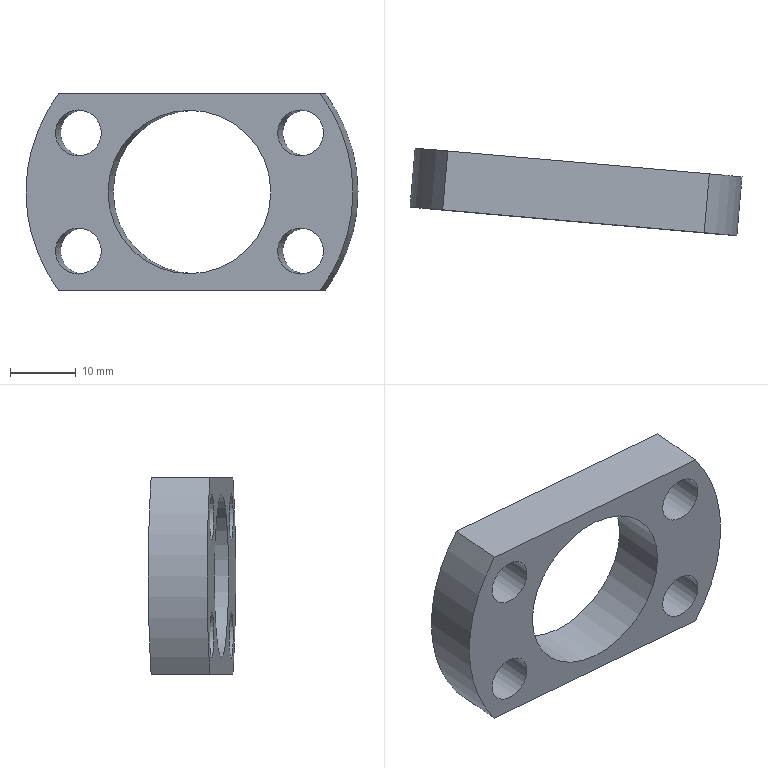Part | NX | features solid 2 | 1 solid | 11 faces | box 50.594 x 13.324 x 30 mm | volume 6871 mm3 | cylinder 7 | plane 4 | commonest cylinder face diameters 7 x4 50 x2 24.9 x1
STEP:
#1=CARTESIAN_POINT('',(318.521,-30.878,-100.));
#2=VERTEX_POINT('',#1);
#3=CARTESIAN_POINT('',(318.521,-30.878,-70.));
#4=VERTEX_POINT('',#3);
#5=CARTESIAN_POINT('',(298.597,-29.135,-85.));
#6=DIRECTION('',(-0.08716,-0.9962,0.));
#7=DIRECTION('',(-0.9962,0.08716,0.));
#8=AXIS2_PLACEMENT_3D('',#5,#6,#7);
#9=CIRCLE('',#8,25.);
#10=EDGE_CURVE('',#2,#4,#9,.T.);
#11=ORIENTED_EDGE('',*,*,#10,.T.);
#12=CARTESIAN_POINT('',(317.736,-39.844,-70.));
#13=VERTEX_POINT('',#12);
#14=CARTESIAN_POINT('',(318.521,-30.878,-70.));
#15=DIRECTION('',(-0.08716,-0.9962,0.));
#16=VECTOR('',#15,1000.);
#17=LINE('',#14,#16);
#18=EDGE_CURVE('',#4,#13,#17,.T.);
#19=ORIENTED_EDGE('',*,*,#18,.T.);
#20=CARTESIAN_POINT('',(317.736,-39.844,-100.));
#21=VERTEX_POINT('',#20);
#22=CARTESIAN_POINT('',(297.813,-38.101,-85.));
#23=DIRECTION('',(-0.08716,-0.9962,0.));
#24=DIRECTION('',(-0.9962,0.08716,0.));
#25=AXIS2_PLACEMENT_3D('',#22,#23,#24);
#26=CIRCLE('',#25,25.);
#27=EDGE_CURVE('',#21,#13,#26,.T.);
#28=ORIENTED_EDGE('',*,*,#27,.F.);
#29=CARTESIAN_POINT('',(318.521,-30.878,-100.));
#30=DIRECTION('',(-0.08716,-0.9962,0.));
#31=VECTOR('',#30,1000.);
#32=LINE('',#29,#31);
#33=EDGE_CURVE('',#2,#21,#32,.T.);
#34=ORIENTED_EDGE('',*,*,#33,.F.);
#35=EDGE_LOOP('',(#11,#19,#28,#34));
#36=FACE_BOUND('',#35,.T.);
#37=CARTESIAN_POINT('',(298.597,-29.135,-85.));
#38=DIRECTION('',(-0.08716,-0.9962,0.));
#39=DIRECTION('',(0.,0.,-1.));
#40=AXIS2_PLACEMENT_3D('',#37,#38,#39);
#41=CYLINDRICAL_SURFACE('',#40,25.);
#42=ADVANCED_FACE('',(#36),#41,.T.);
#43=CARTESIAN_POINT('',(277.889,-36.358,-70.));
#44=VERTEX_POINT('',#43);
#45=CARTESIAN_POINT('',(277.889,-36.358,-100.));
#46=VERTEX_POINT('',#45);
#47=CARTESIAN_POINT('',(297.813,-38.101,-85.));
#48=DIRECTION('',(-0.08716,-0.9962,0.));
#49=DIRECTION('',(-0.9962,0.08716,0.));
#50=AXIS2_PLACEMENT_3D('',#47,#48,#49);
#51=CIRCLE('',#50,25.);
#52=EDGE_CURVE('',#44,#46,#51,.T.);
#53=ORIENTED_EDGE('',*,*,#52,.F.);
#54=CARTESIAN_POINT('',(278.673,-27.392,-70.));
#55=VERTEX_POINT('',#54);
#56=CARTESIAN_POINT('',(278.673,-27.392,-70.));
#57=DIRECTION('',(-0.08716,-0.9962,0.));
#58=VECTOR('',#57,1000.);
#59=LINE('',#56,#58);
#60=EDGE_CURVE('',#44,#55,#59,.F.);
#61=ORIENTED_EDGE('',*,*,#60,.T.);
#62=CARTESIAN_POINT('',(278.673,-27.392,-100.));
#63=VERTEX_POINT('',#62);
#64=CARTESIAN_POINT('',(298.597,-29.135,-85.));
#65=DIRECTION('',(-0.08716,-0.9962,0.));
#66=DIRECTION('',(-0.9962,0.08716,0.));
#67=AXIS2_PLACEMENT_3D('',#64,#65,#66);
#68=CIRCLE('',#67,25.);
#69=EDGE_CURVE('',#55,#63,#68,.T.);
#70=ORIENTED_EDGE('',*,*,#69,.T.);
#71=CARTESIAN_POINT('',(278.673,-27.392,-100.));
#72=DIRECTION('',(-0.08716,-0.9962,0.));
#73=VECTOR('',#72,1000.);
#74=LINE('',#71,#73);
#75=EDGE_CURVE('',#46,#63,#74,.F.);
#76=ORIENTED_EDGE('',*,*,#75,.F.);
#77=EDGE_LOOP('',(#53,#61,#70,#76));
#78=FACE_BOUND('',#77,.T.);
#79=CARTESIAN_POINT('',(298.597,-29.135,-85.));
#80=DIRECTION('',(-0.08716,-0.9962,0.));
#81=DIRECTION('',(0.,0.,-1.));
#82=AXIS2_PLACEMENT_3D('',#79,#80,#81);
#83=CYLINDRICAL_SURFACE('',#82,25.);
#84=ADVANCED_FACE('',(#78),#83,.T.);
#85=CARTESIAN_POINT('',(315.532,-30.617,-90.5));
#86=VERTEX_POINT('',#85);
#87=CARTESIAN_POINT('',(315.532,-30.617,-94.));
#88=DIRECTION('',(-0.08716,-0.9962,0.));
#89=DIRECTION('',(0.,0.,1.));
#90=AXIS2_PLACEMENT_3D('',#87,#88,#89);
#91=CIRCLE('',#90,3.5);
#92=EDGE_CURVE('',#86,#86,#91,.T.);
#93=ORIENTED_EDGE('',*,*,#92,.T.);
#94=EDGE_LOOP('',(#93));
#95=FACE_BOUND('',#94,.T.);
#96=CARTESIAN_POINT('',(315.532,-30.617,-72.5));
#97=VERTEX_POINT('',#96);
#98=CARTESIAN_POINT('',(315.532,-30.617,-76.));
#99=DIRECTION('',(-0.08716,-0.9962,0.));
#100=DIRECTION('',(0.,0.,1.));
#101=AXIS2_PLACEMENT_3D('',#98,#99,#100);
#102=CIRCLE('',#101,3.5);
#103=EDGE_CURVE('',#97,#97,#102,.T.);
#104=ORIENTED_EDGE('',*,*,#103,.T.);
#105=EDGE_LOOP('',(#104));
#106=FACE_BOUND('',#105,.T.);
#107=CARTESIAN_POINT('',(281.662,-27.654,-90.5));
#108=VERTEX_POINT('',#107);
#109=CARTESIAN_POINT('',(281.662,-27.654,-94.));
#110=DIRECTION('',(-0.08716,-0.9962,0.));
#111=DIRECTION('',(0.,0.,1.));
#112=AXIS2_PLACEMENT_3D('',#109,#110,#111);
#113=CIRCLE('',#112,3.5);
#114=EDGE_CURVE('',#108,#108,#113,.T.);
#115=ORIENTED_EDGE('',*,*,#114,.T.);
#116=EDGE_LOOP('',(#115));
#117=FACE_BOUND('',#116,.T.);
#118=CARTESIAN_POINT('',(281.662,-27.654,-72.5));
#119=VERTEX_POINT('',#118);
#120=CARTESIAN_POINT('',(281.662,-27.654,-76.));
#121=DIRECTION('',(-0.08716,-0.9962,0.));
#122=DIRECTION('',(0.,0.,1.));
#123=AXIS2_PLACEMENT_3D('',#120,#121,#122);
#124=CIRCLE('',#123,3.5);
#125=EDGE_CURVE('',#119,#119,#124,.T.);
#126=ORIENTED_EDGE('',*,*,#125,.T.);
#127=EDGE_LOOP('',(#126));
#128=FACE_BOUND('',#127,.T.);
#129=CARTESIAN_POINT('',(298.597,-29.135,-72.55));
#130=VERTEX_POINT('',#129);
#131=CARTESIAN_POINT('',(298.597,-29.135,-85.));
#132=DIRECTION('',(-0.08716,-0.9962,0.));
#133=DIRECTION('',(0.,0.,1.));
#134=AXIS2_PLACEMENT_3D('',#131,#132,#133);
#135=CIRCLE('',#134,12.45);
#136=EDGE_CURVE('',#130,#130,#135,.T.);
#137=ORIENTED_EDGE('',*,*,#136,.T.);
#138=EDGE_LOOP('',(#137));
#139=FACE_BOUND('',#138,.T.);
#140=ORIENTED_EDGE('',*,*,#69,.F.);
#141=CARTESIAN_POINT('',(298.597,-29.135,-70.));
#142=DIRECTION('',(-0.9962,0.08716,0.));
#143=VECTOR('',#142,1000.);
#144=LINE('',#141,#143);
#145=EDGE_CURVE('',#4,#55,#144,.T.);
#146=ORIENTED_EDGE('',*,*,#145,.F.);
#147=ORIENTED_EDGE('',*,*,#10,.F.);
#148=CARTESIAN_POINT('',(298.597,-29.135,-100.));
#149=DIRECTION('',(-0.9962,0.08716,0.));
#150=VECTOR('',#149,1000.);
#151=LINE('',#148,#150);
#152=EDGE_CURVE('',#2,#63,#151,.T.);
#153=ORIENTED_EDGE('',*,*,#152,.T.);
#154=EDGE_LOOP('',(#140,#146,#147,#153));
#155=FACE_BOUND('',#154,.T.);
#156=CARTESIAN_POINT('',(298.597,-29.135,-85.));
#157=DIRECTION('',(0.08716,0.9962,0.));
#158=DIRECTION('',(0.,0.,1.));
#159=AXIS2_PLACEMENT_3D('',#156,#157,#158);
#160=PLANE('',#159);
#161=ADVANCED_FACE('',(#95,#106,#117,#128,#139,#155),#160,.T.);
#162=CARTESIAN_POINT('',(314.748,-39.583,-90.5));
#163=VERTEX_POINT('',#162);
#164=CARTESIAN_POINT('',(314.748,-39.583,-94.));
#165=DIRECTION('',(-0.08716,-0.9962,0.));
#166=DIRECTION('',(0.,0.,1.));
#167=AXIS2_PLACEMENT_3D('',#164,#165,#166);
#168=CIRCLE('',#167,3.5);
#169=EDGE_CURVE('',#163,#163,#168,.T.);
#170=ORIENTED_EDGE('',*,*,#169,.F.);
#171=EDGE_LOOP('',(#170));
#172=FACE_BOUND('',#171,.T.);
#173=CARTESIAN_POINT('',(314.748,-39.583,-72.5));
#174=VERTEX_POINT('',#173);
#175=CARTESIAN_POINT('',(314.748,-39.583,-76.));
#176=DIRECTION('',(-0.08716,-0.9962,0.));
#177=DIRECTION('',(0.,0.,1.));
#178=AXIS2_PLACEMENT_3D('',#175,#176,#177);
#179=CIRCLE('',#178,3.5);
#180=EDGE_CURVE('',#174,#174,#179,.T.);
#181=ORIENTED_EDGE('',*,*,#180,.F.);
#182=EDGE_LOOP('',(#181));
#183=FACE_BOUND('',#182,.T.);
#184=CARTESIAN_POINT('',(280.877,-36.619,-90.5));
#185=VERTEX_POINT('',#184);
#186=CARTESIAN_POINT('',(280.877,-36.619,-94.));
#187=DIRECTION('',(-0.08716,-0.9962,0.));
#188=DIRECTION('',(0.,0.,1.));
#189=AXIS2_PLACEMENT_3D('',#186,#187,#188);
#190=CIRCLE('',#189,3.5);
#191=EDGE_CURVE('',#185,#185,#190,.T.);
#192=ORIENTED_EDGE('',*,*,#191,.F.);
#193=EDGE_LOOP('',(#192));
#194=FACE_BOUND('',#193,.T.);
#195=CARTESIAN_POINT('',(280.877,-36.619,-72.5));
#196=VERTEX_POINT('',#195);
#197=CARTESIAN_POINT('',(280.877,-36.619,-76.));
#198=DIRECTION('',(-0.08716,-0.9962,0.));
#199=DIRECTION('',(0.,0.,1.));
#200=AXIS2_PLACEMENT_3D('',#197,#198,#199);
#201=CIRCLE('',#200,3.5);
#202=EDGE_CURVE('',#196,#196,#201,.T.);
#203=ORIENTED_EDGE('',*,*,#202,.F.);
#204=EDGE_LOOP('',(#203));
#205=FACE_BOUND('',#204,.T.);
#206=CARTESIAN_POINT('',(297.813,-38.101,-72.55));
#207=VERTEX_POINT('',#206);
#208=CARTESIAN_POINT('',(297.813,-38.101,-85.));
#209=DIRECTION('',(-0.08716,-0.9962,0.));
#210=DIRECTION('',(0.,0.,1.));
#211=AXIS2_PLACEMENT_3D('',#208,#209,#210);
#212=CIRCLE('',#211,12.45);
#213=EDGE_CURVE('',#207,#207,#212,.T.);
#214=ORIENTED_EDGE('',*,*,#213,.F.);
#215=EDGE_LOOP('',(#214));
#216=FACE_BOUND('',#215,.T.);
#217=ORIENTED_EDGE('',*,*,#27,.T.);
#218=CARTESIAN_POINT('',(297.813,-38.101,-70.));
#219=DIRECTION('',(-0.9962,0.08716,0.));
#220=VECTOR('',#219,1000.);
#221=LINE('',#218,#220);
#222=EDGE_CURVE('',#13,#44,#221,.T.);
#223=ORIENTED_EDGE('',*,*,#222,.T.);
#224=ORIENTED_EDGE('',*,*,#52,.T.);
#225=CARTESIAN_POINT('',(297.813,-38.101,-100.));
#226=DIRECTION('',(-0.9962,0.08716,0.));
#227=VECTOR('',#226,1000.);
#228=LINE('',#225,#227);
#229=EDGE_CURVE('',#21,#46,#228,.T.);
#230=ORIENTED_EDGE('',*,*,#229,.F.);
#231=EDGE_LOOP('',(#217,#223,#224,#230));
#232=FACE_BOUND('',#231,.T.);
#233=CARTESIAN_POINT('',(297.813,-38.101,-85.));
#234=DIRECTION('',(0.08716,0.9962,0.));
#235=DIRECTION('',(0.,0.,1.));
#236=AXIS2_PLACEMENT_3D('',#233,#234,#235);
#237=PLANE('',#236);
#238=ADVANCED_FACE('',(#172,#183,#194,#205,#216,#232),#237,.F.);
#239=ORIENTED_EDGE('',*,*,#145,.T.);
#240=ORIENTED_EDGE('',*,*,#60,.F.);
#241=ORIENTED_EDGE('',*,*,#222,.F.);
#242=ORIENTED_EDGE('',*,*,#18,.F.);
#243=EDGE_LOOP('',(#239,#240,#241,#242));
#244=FACE_BOUND('',#243,.T.);
#245=CARTESIAN_POINT('',(385.07,-45.735,-70.));
#246=DIRECTION('',(0.,0.,1.));
#247=DIRECTION('',(-0.9962,0.08716,0.));
#248=AXIS2_PLACEMENT_3D('',#245,#246,#247);
#249=PLANE('',#248);
#250=ADVANCED_FACE('',(#244),#249,.T.);
#251=ORIENTED_EDGE('',*,*,#152,.F.);
#252=ORIENTED_EDGE('',*,*,#33,.T.);
#253=ORIENTED_EDGE('',*,*,#229,.T.);
#254=ORIENTED_EDGE('',*,*,#75,.T.);
#255=EDGE_LOOP('',(#251,#252,#253,#254));
#256=FACE_BOUND('',#255,.T.);
#257=CARTESIAN_POINT('',(385.07,-45.735,-100.));
#258=DIRECTION('',(0.,0.,1.));
#259=DIRECTION('',(-0.9962,0.08716,0.));
#260=AXIS2_PLACEMENT_3D('',#257,#258,#259);
#261=PLANE('',#260);
#262=ADVANCED_FACE('',(#256),#261,.F.);
#263=ORIENTED_EDGE('',*,*,#136,.F.);
#264=EDGE_LOOP('',(#263));
#265=FACE_BOUND('',#264,.T.);
#266=ORIENTED_EDGE('',*,*,#213,.T.);
#267=EDGE_LOOP('',(#266));
#268=FACE_BOUND('',#267,.T.);
#269=CARTESIAN_POINT('',(264.432,-419.644,-85.));
#270=DIRECTION('',(0.08716,0.9962,0.));
#271=DIRECTION('',(0.,0.,1.));
#272=AXIS2_PLACEMENT_3D('',#269,#270,#271);
#273=CYLINDRICAL_SURFACE('',#272,12.45);
#274=ADVANCED_FACE('',(#265,#268),#273,.F.);
#275=ORIENTED_EDGE('',*,*,#125,.F.);
#276=EDGE_LOOP('',(#275));
#277=FACE_BOUND('',#276,.T.);
#278=ORIENTED_EDGE('',*,*,#202,.T.);
#279=EDGE_LOOP('',(#278));
#280=FACE_BOUND('',#279,.T.);
#281=CARTESIAN_POINT('',(278.263,-66.505,-76.));
#282=DIRECTION('',(0.08716,0.9962,0.));
#283=DIRECTION('',(0.9962,-0.08716,0.));
#284=AXIS2_PLACEMENT_3D('',#281,#282,#283);
#285=CYLINDRICAL_SURFACE('',#284,3.5);
#286=ADVANCED_FACE('',(#277,#280),#285,.F.);
#287=ORIENTED_EDGE('',*,*,#114,.F.);
#288=EDGE_LOOP('',(#287));
#289=FACE_BOUND('',#288,.T.);
#290=ORIENTED_EDGE('',*,*,#191,.T.);
#291=EDGE_LOOP('',(#290));
#292=FACE_BOUND('',#291,.T.);
#293=CARTESIAN_POINT('',(278.263,-66.505,-94.));
#294=DIRECTION('',(0.08716,0.9962,0.));
#295=DIRECTION('',(0.9962,-0.08716,0.));
#296=AXIS2_PLACEMENT_3D('',#293,#294,#295);
#297=CYLINDRICAL_SURFACE('',#296,3.5);
#298=ADVANCED_FACE('',(#289,#292),#297,.F.);
#299=ORIENTED_EDGE('',*,*,#103,.F.);
#300=EDGE_LOOP('',(#299));
#301=FACE_BOUND('',#300,.T.);
#302=ORIENTED_EDGE('',*,*,#180,.T.);
#303=EDGE_LOOP('',(#302));
#304=FACE_BOUND('',#303,.T.);
#305=CARTESIAN_POINT('',(312.133,-69.469,-76.));
#306=DIRECTION('',(0.08716,0.9962,0.));
#307=DIRECTION('',(0.,0.,1.));
#308=AXIS2_PLACEMENT_3D('',#305,#306,#307);
#309=CYLINDRICAL_SURFACE('',#308,3.5);
#310=ADVANCED_FACE('',(#301,#304),#309,.F.);
#311=ORIENTED_EDGE('',*,*,#92,.F.);
#312=EDGE_LOOP('',(#311));
#313=FACE_BOUND('',#312,.T.);
#314=ORIENTED_EDGE('',*,*,#169,.T.);
#315=EDGE_LOOP('',(#314));
#316=FACE_BOUND('',#315,.T.);
#317=CARTESIAN_POINT('',(312.133,-69.469,-94.));
#318=DIRECTION('',(0.08716,0.9962,0.));
#319=DIRECTION('',(0.,0.,1.));
#320=AXIS2_PLACEMENT_3D('',#317,#318,#319);
#321=CYLINDRICAL_SURFACE('',#320,3.5);
#322=ADVANCED_FACE('',(#313,#316),#321,.F.);
#323=CLOSED_SHELL('',(#42,#84,#161,#238,#250,#262,#274,#286,#298,#310,#322));
#324=MANIFOLD_SOLID_BREP('',#323);
#325=(LENGTH_UNIT()NAMED_UNIT(*)SI_UNIT(.MILLI.,.METRE.));
#326=UNCERTAINTY_MEASURE_WITH_UNIT(LENGTH_MEASURE(0.00001),#325,'','');
#327=(NAMED_UNIT(*)PLANE_ANGLE_UNIT()SI_UNIT($,.RADIAN.));
#328=(NAMED_UNIT(*)SI_UNIT($,.STERADIAN.)SOLID_ANGLE_UNIT());
#329=(GEOMETRIC_REPRESENTATION_CONTEXT(3)GLOBAL_UNCERTAINTY_ASSIGNED_CONTEXT((#326))GLOBAL_UNIT_ASSIGNED_CONTEXT((#325,#327,#328))REPRESENTATION_CONTEXT('',''));
#330=ADVANCED_BREP_SHAPE_REPRESENTATION('',(#324),#329);